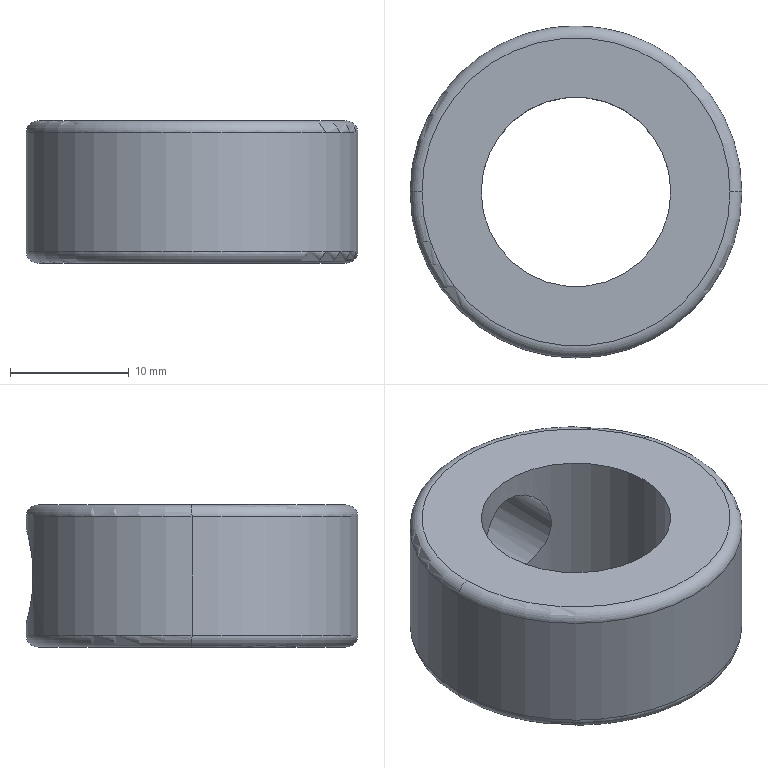Part | SolidWorks | features Extrusion 1, Fillet 1, ICE 1 | 1 solid | 12 faces | box 28 x 28 x 12 mm | volume 4632 mm3 | cylinder 6 | torus 4 | plane 2 | commonest cylinder face diameters 8 x2 16 x2 28 x2
STEP:
#1=CARTESIAN_POINT('',(0.,14.,-4.));
#2=VERTEX_POINT('',#1);
#3=CARTESIAN_POINT('',(0.,14.,4.));
#4=VERTEX_POINT('',#3);
#5=CARTESIAN_POINT('',(0.,14.,-4.));
#6=CARTESIAN_POINT('',(-0.2658,14.,-4.));
#7=CARTESIAN_POINT('',(-0.5269,13.992,-3.974));
#8=CARTESIAN_POINT('',(-1.04,13.964,-3.871));
#9=CARTESIAN_POINT('',(-1.295,13.942,-3.794));
#10=CARTESIAN_POINT('',(-1.779,13.889,-3.592));
#11=CARTESIAN_POINT('',(-2.008,13.857,-3.469));
#12=CARTESIAN_POINT('',(-2.442,13.787,-3.179));
#13=CARTESIAN_POINT('',(-2.646,13.749,-3.011));
#14=CARTESIAN_POINT('',(-3.013,13.673,-2.644));
#15=CARTESIAN_POINT('',(-3.178,13.635,-2.443));
#16=CARTESIAN_POINT('',(-3.47,13.564,-2.007));
#17=CARTESIAN_POINT('',(-3.594,13.531,-1.776));
#18=CARTESIAN_POINT('',(-3.793,13.477,-1.295));
#19=CARTESIAN_POINT('',(-3.871,13.454,-1.042));
#20=CARTESIAN_POINT('',(-3.974,13.424,-0.5247));
#21=CARTESIAN_POINT('',(-4.,13.416,-0.2642));
#22=CARTESIAN_POINT('',(-4.,13.416,0.2607));
#23=CARTESIAN_POINT('',(-3.974,13.424,0.5273));
#24=CARTESIAN_POINT('',(-3.871,13.454,1.042));
#25=CARTESIAN_POINT('',(-3.795,13.476,1.292));
#26=CARTESIAN_POINT('',(-3.593,13.532,1.778));
#27=CARTESIAN_POINT('',(-3.468,13.564,2.009));
#28=CARTESIAN_POINT('',(-3.179,13.635,2.441));
#29=CARTESIAN_POINT('',(-3.012,13.673,2.645));
#30=CARTESIAN_POINT('',(-2.643,13.75,3.014));
#31=CARTESIAN_POINT('',(-2.442,13.787,3.179));
#32=CARTESIAN_POINT('',(-2.01,13.857,3.468));
#33=CARTESIAN_POINT('',(-1.776,13.889,3.594));
#34=CARTESIAN_POINT('',(-1.293,13.942,3.794));
#35=CARTESIAN_POINT('',(-1.044,13.963,3.87));
#36=CARTESIAN_POINT('',(-0.5274,13.992,3.974));
#37=CARTESIAN_POINT('',(-0.2619,14.,4.));
#38=CARTESIAN_POINT('',(0.,14.,4.));
#39=B_SPLINE_CURVE_WITH_KNOTS('',3,(#5,#6,#7,#8,#9,#10,#11,#12,#13,#14,#15,#16,#17,#18,#19,#20,#21,#22,#23,#24,#25,#26,#27,#28,#29,#30,#31,#32,#33,#34,#35,#36,#37,#38),.UNSPECIFIED.,.F.,.F.,(4,2,2,2,2,2,2,2,2,2,2,2,2,2,2,2,4),(0.,0.0007857,0.001571,0.002357,0.003143,0.003929,0.004714,0.0055,0.006286,0.007072,0.007857,0.008643,0.009429,0.01021,0.011,0.01179,0.01257),.UNSPECIFIED.);
#40=EDGE_CURVE('',#2,#4,#39,.T.);
#41=ORIENTED_EDGE('',*,*,#40,.T.);
#42=CARTESIAN_POINT('',(0.,8.,4.));
#43=VERTEX_POINT('',#42);
#44=CARTESIAN_POINT('',(0.,20.,4.));
#45=DIRECTION('',(0.,-1.,0.));
#46=VECTOR('',#45,1000.);
#47=LINE('',#44,#46);
#48=EDGE_CURVE('',#4,#43,#47,.T.);
#49=ORIENTED_EDGE('',*,*,#48,.T.);
#50=CARTESIAN_POINT('',(0.,8.,-4.));
#51=VERTEX_POINT('',#50);
#52=CARTESIAN_POINT('',(0.,8.,-4.));
#53=CARTESIAN_POINT('',(-0.2692,8.,-4.));
#54=CARTESIAN_POINT('',(-0.5331,7.986,-3.973));
#55=CARTESIAN_POINT('',(-1.051,7.935,-3.869));
#56=CARTESIAN_POINT('',(-1.307,7.896,-3.789));
#57=CARTESIAN_POINT('',(-1.79,7.801,-3.587));
#58=CARTESIAN_POINT('',(-2.019,7.744,-3.463));
#59=CARTESIAN_POINT('',(-2.45,7.619,-3.172));
#60=CARTESIAN_POINT('',(-2.65,7.551,-3.007));
#61=CARTESIAN_POINT('',(-3.013,7.414,-2.644));
#62=CARTESIAN_POINT('',(-3.178,7.344,-2.443));
#63=CARTESIAN_POINT('',(-3.466,7.212,-2.013));
#64=CARTESIAN_POINT('',(-3.589,7.151,-1.786));
#65=CARTESIAN_POINT('',(-3.789,7.046,-1.307));
#66=CARTESIAN_POINT('',(-3.869,7.003,-1.051));
#67=CARTESIAN_POINT('',(-3.973,6.944,-0.5326));
#68=CARTESIAN_POINT('',(-4.,6.928,-0.2701));
#69=CARTESIAN_POINT('',(-4.,6.928,0.2623));
#70=CARTESIAN_POINT('',(-3.973,6.944,0.532));
#71=CARTESIAN_POINT('',(-3.869,7.003,1.05));
#72=CARTESIAN_POINT('',(-3.791,7.046,1.304));
#73=CARTESIAN_POINT('',(-3.588,7.151,1.788));
#74=CARTESIAN_POINT('',(-3.465,7.213,2.016));
#75=CARTESIAN_POINT('',(-3.176,7.344,2.445));
#76=CARTESIAN_POINT('',(-3.01,7.415,2.647));
#77=CARTESIAN_POINT('',(-2.647,7.552,3.01));
#78=CARTESIAN_POINT('',(-2.449,7.619,3.173));
#79=CARTESIAN_POINT('',(-2.016,7.745,3.465));
#80=CARTESIAN_POINT('',(-1.786,7.802,3.588));
#81=CARTESIAN_POINT('',(-1.306,7.896,3.79));
#82=CARTESIAN_POINT('',(-1.052,7.935,3.868));
#83=CARTESIAN_POINT('',(-0.5291,7.987,3.974));
#84=CARTESIAN_POINT('',(-0.2656,8.,4.));
#85=CARTESIAN_POINT('',(0.,8.,4.));
#86=B_SPLINE_CURVE_WITH_KNOTS('',3,(#52,#53,#54,#55,#56,#57,#58,#59,#60,#61,#62,#63,#64,#65,#66,#67,#68,#69,#70,#71,#72,#73,#74,#75,#76,#77,#78,#79,#80,#81,#82,#83,#84,#85),.UNSPECIFIED.,.F.,.F.,(4,2,2,2,2,2,2,2,2,2,2,2,2,2,2,2,4),(0.,0.0007952,0.00159,0.002386,0.003181,0.003976,0.004771,0.005567,0.006362,0.007157,0.007952,0.008748,0.009543,0.01034,0.01113,0.01193,0.01272),.UNSPECIFIED.);
#87=EDGE_CURVE('',#51,#43,#86,.T.);
#88=ORIENTED_EDGE('',*,*,#87,.F.);
#89=CARTESIAN_POINT('',(0.,20.,-4.));
#90=DIRECTION('',(0.,-1.,0.));
#91=VECTOR('',#90,1000.);
#92=LINE('',#89,#91);
#93=EDGE_CURVE('',#2,#51,#92,.T.);
#94=ORIENTED_EDGE('',*,*,#93,.F.);
#95=EDGE_LOOP('',(#41,#49,#88,#94));
#96=FACE_OUTER_BOUND('',#95,.T.);
#97=CARTESIAN_POINT('',(0.,20.,0.));
#98=DIRECTION('',(0.,-1.,0.));
#99=DIRECTION('',(0.,0.,-1.));
#100=AXIS2_PLACEMENT_3D('',#97,#98,#99);
#101=CYLINDRICAL_SURFACE('',#100,4.);
#102=ADVANCED_FACE('',(#96),#101,.F.);
#103=CARTESIAN_POINT('',(-14.,0.,5.));
#104=VERTEX_POINT('',#103);
#105=CARTESIAN_POINT('',(14.,0.,5.));
#106=VERTEX_POINT('',#105);
#107=CARTESIAN_POINT('',(0.,0.,5.));
#108=DIRECTION('',(0.,0.,-1.));
#109=DIRECTION('',(1.,0.,0.));
#110=AXIS2_PLACEMENT_3D('',#107,#108,#109);
#111=CIRCLE('',#110,14.);
#112=EDGE_CURVE('',#104,#106,#111,.T.);
#113=ORIENTED_EDGE('',*,*,#112,.F.);
#114=CARTESIAN_POINT('',(-13.,0.,6.));
#115=VERTEX_POINT('',#114);
#116=CARTESIAN_POINT('',(-13.,0.,5.));
#117=DIRECTION('',(0.,1.,0.));
#118=DIRECTION('',(-1.,0.,0.));
#119=AXIS2_PLACEMENT_3D('',#116,#117,#118);
#120=CIRCLE('',#119,1.);
#121=EDGE_CURVE('',#104,#115,#120,.T.);
#122=ORIENTED_EDGE('',*,*,#121,.T.);
#123=CARTESIAN_POINT('',(13.,0.,6.));
#124=VERTEX_POINT('',#123);
#125=CARTESIAN_POINT('',(0.,0.,6.));
#126=DIRECTION('',(0.,0.,1.));
#127=DIRECTION('',(1.,0.,0.));
#128=AXIS2_PLACEMENT_3D('',#125,#126,#127);
#129=CIRCLE('',#128,13.);
#130=EDGE_CURVE('',#124,#115,#129,.T.);
#131=ORIENTED_EDGE('',*,*,#130,.F.);
#132=CARTESIAN_POINT('',(13.,0.,5.));
#133=DIRECTION('',(0.,-1.,0.));
#134=DIRECTION('',(0.,0.,-1.));
#135=AXIS2_PLACEMENT_3D('',#132,#133,#134);
#136=CIRCLE('',#135,1.);
#137=EDGE_CURVE('',#106,#124,#136,.T.);
#138=ORIENTED_EDGE('',*,*,#137,.F.);
#139=EDGE_LOOP('',(#113,#122,#131,#138));
#140=FACE_OUTER_BOUND('',#139,.T.);
#141=CARTESIAN_POINT('',(0.,0.,5.));
#142=DIRECTION('',(0.,0.,1.));
#143=DIRECTION('',(1.,0.,0.));
#144=AXIS2_PLACEMENT_3D('',#141,#142,#143);
#145=TOROIDAL_SURFACE('',#144,13.,1.);
#146=ADVANCED_FACE('',(#140),#145,.T.);
#147=CARTESIAN_POINT('',(-13.,0.,-6.));
#148=VERTEX_POINT('',#147);
#149=CARTESIAN_POINT('',(13.,0.,-6.));
#150=VERTEX_POINT('',#149);
#151=CARTESIAN_POINT('',(0.,0.,-6.));
#152=DIRECTION('',(0.,0.,-1.));
#153=DIRECTION('',(1.,0.,0.));
#154=AXIS2_PLACEMENT_3D('',#151,#152,#153);
#155=CIRCLE('',#154,13.);
#156=EDGE_CURVE('',#148,#150,#155,.T.);
#157=ORIENTED_EDGE('',*,*,#156,.F.);
#158=CARTESIAN_POINT('',(-14.,0.,-5.));
#159=VERTEX_POINT('',#158);
#160=CARTESIAN_POINT('',(-13.,0.,-5.));
#161=DIRECTION('',(0.,1.,0.));
#162=DIRECTION('',(-1.,0.,0.));
#163=AXIS2_PLACEMENT_3D('',#160,#161,#162);
#164=CIRCLE('',#163,1.);
#165=EDGE_CURVE('',#148,#159,#164,.T.);
#166=ORIENTED_EDGE('',*,*,#165,.T.);
#167=CARTESIAN_POINT('',(14.,0.,-5.));
#168=VERTEX_POINT('',#167);
#169=CARTESIAN_POINT('',(0.,0.,-5.));
#170=DIRECTION('',(0.,0.,1.));
#171=DIRECTION('',(1.,0.,0.));
#172=AXIS2_PLACEMENT_3D('',#169,#170,#171);
#173=CIRCLE('',#172,14.);
#174=EDGE_CURVE('',#168,#159,#173,.T.);
#175=ORIENTED_EDGE('',*,*,#174,.F.);
#176=CARTESIAN_POINT('',(13.,0.,-5.));
#177=DIRECTION('',(0.,-1.,0.));
#178=DIRECTION('',(0.,0.,-1.));
#179=AXIS2_PLACEMENT_3D('',#176,#177,#178);
#180=CIRCLE('',#179,1.);
#181=EDGE_CURVE('',#150,#168,#180,.T.);
#182=ORIENTED_EDGE('',*,*,#181,.F.);
#183=EDGE_LOOP('',(#157,#166,#175,#182));
#184=FACE_OUTER_BOUND('',#183,.T.);
#185=CARTESIAN_POINT('',(0.,0.,-5.));
#186=DIRECTION('',(0.,0.,1.));
#187=DIRECTION('',(1.,0.,0.));
#188=AXIS2_PLACEMENT_3D('',#185,#186,#187);
#189=TOROIDAL_SURFACE('',#188,13.,1.);
#190=ADVANCED_FACE('',(#184),#189,.T.);
#191=CARTESIAN_POINT('',(-8.,0.,6.));
#192=VERTEX_POINT('',#191);
#193=CARTESIAN_POINT('',(8.,0.,6.));
#194=VERTEX_POINT('',#193);
#195=CARTESIAN_POINT('',(0.,0.,6.));
#196=DIRECTION('',(0.,0.,1.));
#197=DIRECTION('',(1.,0.,0.));
#198=AXIS2_PLACEMENT_3D('',#195,#196,#197);
#199=CIRCLE('',#198,8.);
#200=EDGE_CURVE('',#192,#194,#199,.T.);
#201=ORIENTED_EDGE('',*,*,#200,.T.);
#202=CARTESIAN_POINT('',(8.,0.,-6.));
#203=VERTEX_POINT('',#202);
#204=CARTESIAN_POINT('',(8.,0.,6.));
#205=DIRECTION('',(0.,0.,-1.));
#206=VECTOR('',#205,1000.);
#207=LINE('',#204,#206);
#208=EDGE_CURVE('',#194,#203,#207,.T.);
#209=ORIENTED_EDGE('',*,*,#208,.T.);
#210=CARTESIAN_POINT('',(-8.,0.,-6.));
#211=VERTEX_POINT('',#210);
#212=CARTESIAN_POINT('',(0.,0.,-6.));
#213=DIRECTION('',(0.,0.,1.));
#214=DIRECTION('',(1.,0.,0.));
#215=AXIS2_PLACEMENT_3D('',#212,#213,#214);
#216=CIRCLE('',#215,8.);
#217=EDGE_CURVE('',#211,#203,#216,.T.);
#218=ORIENTED_EDGE('',*,*,#217,.F.);
#219=CARTESIAN_POINT('',(-8.,0.,6.));
#220=DIRECTION('',(0.,0.,-1.));
#221=VECTOR('',#220,1000.);
#222=LINE('',#219,#221);
#223=EDGE_CURVE('',#192,#211,#222,.T.);
#224=ORIENTED_EDGE('',*,*,#223,.F.);
#225=EDGE_LOOP('',(#201,#209,#218,#224));
#226=FACE_OUTER_BOUND('',#225,.T.);
#227=CARTESIAN_POINT('',(0.,0.,6.));
#228=DIRECTION('',(0.,0.,-1.));
#229=DIRECTION('',(-1.,0.,0.));
#230=AXIS2_PLACEMENT_3D('',#227,#228,#229);
#231=CYLINDRICAL_SURFACE('',#230,8.);
#232=ADVANCED_FACE('',(#226),#231,.F.);
#233=ORIENTED_EDGE('',*,*,#40,.F.);
#234=CARTESIAN_POINT('',(0.,14.,4.));
#235=CARTESIAN_POINT('',(0.2619,14.,4.));
#236=CARTESIAN_POINT('',(0.524,13.993,3.974));
#237=CARTESIAN_POINT('',(1.043,13.963,3.871));
#238=CARTESIAN_POINT('',(1.294,13.942,3.794));
#239=CARTESIAN_POINT('',(1.776,13.889,3.594));
#240=CARTESIAN_POINT('',(2.01,13.857,3.468));
#241=CARTESIAN_POINT('',(2.443,13.787,3.178));
#242=CARTESIAN_POINT('',(2.643,13.749,3.013));
#243=CARTESIAN_POINT('',(3.012,13.673,2.645));
#244=CARTESIAN_POINT('',(3.18,13.635,2.441));
#245=CARTESIAN_POINT('',(3.468,13.564,2.009));
#246=CARTESIAN_POINT('',(3.592,13.532,1.78));
#247=CARTESIAN_POINT('',(3.795,13.476,1.292));
#248=CARTESIAN_POINT('',(3.871,13.454,1.042));
#249=CARTESIAN_POINT('',(3.973,13.424,0.5296));
#250=CARTESIAN_POINT('',(4.,13.416,0.2643));
#251=CARTESIAN_POINT('',(4.,13.416,-0.2631));
#252=CARTESIAN_POINT('',(3.974,13.424,-0.5236));
#253=CARTESIAN_POINT('',(3.872,13.454,-1.038));
#254=CARTESIAN_POINT('',(3.794,13.477,-1.294));
#255=CARTESIAN_POINT('',(3.594,13.531,-1.776));
#256=CARTESIAN_POINT('',(3.471,13.564,-2.005));
#257=CARTESIAN_POINT('',(3.179,13.635,-2.442));
#258=CARTESIAN_POINT('',(3.013,13.673,-2.644));
#259=CARTESIAN_POINT('',(2.646,13.749,-3.011));
#260=CARTESIAN_POINT('',(2.443,13.787,-3.178));
#261=CARTESIAN_POINT('',(2.008,13.857,-3.469));
#262=CARTESIAN_POINT('',(1.779,13.889,-3.592));
#263=CARTESIAN_POINT('',(1.297,13.942,-3.793));
#264=CARTESIAN_POINT('',(1.042,13.964,-3.871));
#265=CARTESIAN_POINT('',(0.5273,13.992,-3.974));
#266=CARTESIAN_POINT('',(0.2657,14.,-4.));
#267=CARTESIAN_POINT('',(0.,14.,-4.));
#268=B_SPLINE_CURVE_WITH_KNOTS('',3,(#234,#235,#236,#237,#238,#239,#240,#241,#242,#243,#244,#245,#246,#247,#248,#249,#250,#251,#252,#253,#254,#255,#256,#257,#258,#259,#260,#261,#262,#263,#264,#265,#266,#267),.UNSPECIFIED.,.F.,.F.,(4,2,2,2,2,2,2,2,2,2,2,2,2,2,2,2,4),(0.01257,0.01336,0.01414,0.01493,0.01571,0.0165,0.01728,0.01807,0.01886,0.01964,0.02043,0.02121,0.022,0.02278,0.02357,0.02435,0.02514),.UNSPECIFIED.);
#269=EDGE_CURVE('',#4,#2,#268,.T.);
#270=ORIENTED_EDGE('',*,*,#269,.F.);
#271=EDGE_LOOP('',(#233,#270));
#272=FACE_BOUND('',#271,.T.);
#273=ORIENTED_EDGE('',*,*,#112,.T.);
#274=CARTESIAN_POINT('',(14.,0.,6.));
#275=DIRECTION('',(0.,0.,-1.));
#276=VECTOR('',#275,1000.);
#277=LINE('',#274,#276);
#278=EDGE_CURVE('',#106,#168,#277,.T.);
#279=ORIENTED_EDGE('',*,*,#278,.T.);
#280=ORIENTED_EDGE('',*,*,#174,.T.);
#281=CARTESIAN_POINT('',(-14.,0.,6.));
#282=DIRECTION('',(0.,0.,-1.));
#283=VECTOR('',#282,1000.);
#284=LINE('',#281,#283);
#285=EDGE_CURVE('',#104,#159,#284,.T.);
#286=ORIENTED_EDGE('',*,*,#285,.F.);
#287=EDGE_LOOP('',(#273,#279,#280,#286));
#288=FACE_OUTER_BOUND('',#287,.T.);
#289=CARTESIAN_POINT('',(0.,0.,6.));
#290=DIRECTION('',(0.,0.,-1.));
#291=DIRECTION('',(-1.,0.,0.));
#292=AXIS2_PLACEMENT_3D('',#289,#290,#291);
#293=CYLINDRICAL_SURFACE('',#292,14.);
#294=ADVANCED_FACE('',(#272,#288),#293,.T.);
#295=ORIENTED_EDGE('',*,*,#278,.F.);
#296=CARTESIAN_POINT('',(0.,0.,5.));
#297=DIRECTION('',(0.,0.,-1.));
#298=DIRECTION('',(1.,0.,0.));
#299=AXIS2_PLACEMENT_3D('',#296,#297,#298);
#300=CIRCLE('',#299,14.);
#301=EDGE_CURVE('',#106,#104,#300,.T.);
#302=ORIENTED_EDGE('',*,*,#301,.T.);
#303=ORIENTED_EDGE('',*,*,#285,.T.);
#304=CARTESIAN_POINT('',(0.,0.,-5.));
#305=DIRECTION('',(0.,0.,1.));
#306=DIRECTION('',(1.,0.,0.));
#307=AXIS2_PLACEMENT_3D('',#304,#305,#306);
#308=CIRCLE('',#307,14.);
#309=EDGE_CURVE('',#159,#168,#308,.T.);
#310=ORIENTED_EDGE('',*,*,#309,.T.);
#311=EDGE_LOOP('',(#295,#302,#303,#310));
#312=FACE_OUTER_BOUND('',#311,.T.);
#313=CARTESIAN_POINT('',(0.,0.,6.));
#314=DIRECTION('',(0.,0.,-1.));
#315=DIRECTION('',(-1.,0.,0.));
#316=AXIS2_PLACEMENT_3D('',#313,#314,#315);
#317=CYLINDRICAL_SURFACE('',#316,14.);
#318=ADVANCED_FACE('',(#312),#317,.T.);
#319=ORIENTED_EDGE('',*,*,#208,.F.);
#320=CARTESIAN_POINT('',(0.,0.,6.));
#321=DIRECTION('',(0.,0.,1.));
#322=DIRECTION('',(1.,0.,0.));
#323=AXIS2_PLACEMENT_3D('',#320,#321,#322);
#324=CIRCLE('',#323,8.);
#325=EDGE_CURVE('',#194,#192,#324,.T.);
#326=ORIENTED_EDGE('',*,*,#325,.T.);
#327=ORIENTED_EDGE('',*,*,#223,.T.);
#328=CARTESIAN_POINT('',(0.,0.,-6.));
#329=DIRECTION('',(0.,0.,1.));
#330=DIRECTION('',(1.,0.,0.));
#331=AXIS2_PLACEMENT_3D('',#328,#329,#330);
#332=CIRCLE('',#331,8.);
#333=EDGE_CURVE('',#203,#211,#332,.T.);
#334=ORIENTED_EDGE('',*,*,#333,.F.);
#335=EDGE_LOOP('',(#319,#326,#327,#334));
#336=FACE_OUTER_BOUND('',#335,.T.);
#337=ORIENTED_EDGE('',*,*,#87,.T.);
#338=CARTESIAN_POINT('',(0.,8.,4.));
#339=CARTESIAN_POINT('',(0.2651,8.,4.));
#340=CARTESIAN_POINT('',(0.5349,7.986,3.973));
#341=CARTESIAN_POINT('',(1.053,7.935,3.868));
#342=CARTESIAN_POINT('',(1.305,7.897,3.79));
#343=CARTESIAN_POINT('',(1.792,7.801,3.586));
#344=CARTESIAN_POINT('',(2.021,7.744,3.462));
#345=CARTESIAN_POINT('',(2.449,7.619,3.173));
#346=CARTESIAN_POINT('',(2.651,7.551,3.006));
#347=CARTESIAN_POINT('',(3.014,7.413,2.642));
#348=CARTESIAN_POINT('',(3.176,7.344,2.445));
#349=CARTESIAN_POINT('',(3.465,7.213,2.016));
#350=CARTESIAN_POINT('',(3.589,7.151,1.785));
#351=CARTESIAN_POINT('',(3.79,7.046,1.306));
#352=CARTESIAN_POINT('',(3.867,7.004,1.057));
#353=CARTESIAN_POINT('',(3.973,6.944,0.5351));
#354=CARTESIAN_POINT('',(4.,6.928,0.2689));
#355=CARTESIAN_POINT('',(4.,6.928,-0.1279));
#356=CARTESIAN_POINT('',(3.994,6.932,-0.2603));
#357=CARTESIAN_POINT('',(3.968,6.947,-0.5254));
#358=CARTESIAN_POINT('',(3.948,6.958,-0.6587));
#359=CARTESIAN_POINT('',(3.869,7.002,-1.049));
#360=CARTESIAN_POINT('',(3.792,7.045,-1.3));
#361=CARTESIAN_POINT('',(3.59,7.15,-1.784));
#362=CARTESIAN_POINT('',(3.465,7.212,-2.014));
#363=CARTESIAN_POINT('',(3.178,7.343,-2.442));
#364=CARTESIAN_POINT('',(3.013,7.413,-2.643));
#365=CARTESIAN_POINT('',(2.649,7.551,-3.009));
#366=CARTESIAN_POINT('',(2.451,7.619,-3.172));
#367=CARTESIAN_POINT('',(2.023,7.743,-3.46));
#368=CARTESIAN_POINT('',(1.79,7.801,-3.587));
#369=CARTESIAN_POINT('',(1.308,7.896,-3.789));
#370=CARTESIAN_POINT('',(1.058,7.934,-3.867));
#371=CARTESIAN_POINT('',(0.5388,7.986,-3.972));
#372=CARTESIAN_POINT('',(0.2687,8.,-4.));
#373=CARTESIAN_POINT('',(0.,8.,-4.));
#374=B_SPLINE_CURVE_WITH_KNOTS('',3,(#338,#339,#340,#341,#342,#343,#344,#345,#346,#347,#348,#349,#350,#351,#352,#353,#354,#355,#356,#357,#358,#359,#360,#361,#362,#363,#364,#365,#366,#367,#368,#369,#370,#371,#372,#373),.UNSPECIFIED.,.F.,.F.,(4,2,2,2,2,2,2,2,2,2,2,2,2,2,2,2,2,4),(0.01272,0.01352,0.01431,0.01511,0.0159,0.01669,0.01749,0.01828,0.01907,0.01947,0.01987,0.02066,0.02146,0.02225,0.02304,0.02384,0.02463,0.02543),.UNSPECIFIED.);
#375=EDGE_CURVE('',#43,#51,#374,.T.);
#376=ORIENTED_EDGE('',*,*,#375,.T.);
#377=EDGE_LOOP('',(#337,#376));
#378=FACE_BOUND('',#377,.T.);
#379=CARTESIAN_POINT('',(0.,0.,6.));
#380=DIRECTION('',(0.,0.,-1.));
#381=DIRECTION('',(-1.,0.,0.));
#382=AXIS2_PLACEMENT_3D('',#379,#380,#381);
#383=CYLINDRICAL_SURFACE('',#382,8.);
#384=ADVANCED_FACE('',(#336,#378),#383,.F.);
#385=ORIENTED_EDGE('',*,*,#130,.T.);
#386=CARTESIAN_POINT('',(0.,0.,6.));
#387=DIRECTION('',(0.,0.,1.));
#388=DIRECTION('',(1.,0.,0.));
#389=AXIS2_PLACEMENT_3D('',#386,#387,#388);
#390=CIRCLE('',#389,13.);
#391=EDGE_CURVE('',#115,#124,#390,.T.);
#392=ORIENTED_EDGE('',*,*,#391,.T.);
#393=EDGE_LOOP('',(#385,#392));
#394=FACE_OUTER_BOUND('',#393,.T.);
#395=ORIENTED_EDGE('',*,*,#200,.F.);
#396=ORIENTED_EDGE('',*,*,#325,.F.);
#397=EDGE_LOOP('',(#395,#396));
#398=FACE_BOUND('',#397,.T.);
#399=CARTESIAN_POINT('',(0.,0.,6.));
#400=DIRECTION('',(0.,0.,1.));
#401=DIRECTION('',(1.,0.,0.));
#402=AXIS2_PLACEMENT_3D('',#399,#400,#401);
#403=PLANE('',#402);
#404=ADVANCED_FACE('',(#394,#398),#403,.T.);
#405=CARTESIAN_POINT('',(0.,0.,-6.));
#406=DIRECTION('',(0.,0.,-1.));
#407=DIRECTION('',(1.,0.,0.));
#408=AXIS2_PLACEMENT_3D('',#405,#406,#407);
#409=CIRCLE('',#408,13.);
#410=EDGE_CURVE('',#150,#148,#409,.T.);
#411=ORIENTED_EDGE('',*,*,#410,.T.);
#412=ORIENTED_EDGE('',*,*,#156,.T.);
#413=EDGE_LOOP('',(#411,#412));
#414=FACE_OUTER_BOUND('',#413,.T.);
#415=ORIENTED_EDGE('',*,*,#217,.T.);
#416=ORIENTED_EDGE('',*,*,#333,.T.);
#417=EDGE_LOOP('',(#415,#416));
#418=FACE_BOUND('',#417,.T.);
#419=CARTESIAN_POINT('',(0.,0.,-6.));
#420=DIRECTION('',(0.,0.,1.));
#421=DIRECTION('',(1.,0.,0.));
#422=AXIS2_PLACEMENT_3D('',#419,#420,#421);
#423=PLANE('',#422);
#424=ADVANCED_FACE('',(#414,#418),#423,.F.);
#425=ORIENTED_EDGE('',*,*,#165,.F.);
#426=ORIENTED_EDGE('',*,*,#410,.F.);
#427=ORIENTED_EDGE('',*,*,#181,.T.);
#428=ORIENTED_EDGE('',*,*,#309,.F.);
#429=EDGE_LOOP('',(#425,#426,#427,#428));
#430=FACE_OUTER_BOUND('',#429,.T.);
#431=CARTESIAN_POINT('',(0.,0.,-5.));
#432=DIRECTION('',(0.,0.,1.));
#433=DIRECTION('',(1.,0.,0.));
#434=AXIS2_PLACEMENT_3D('',#431,#432,#433);
#435=TOROIDAL_SURFACE('',#434,13.,1.);
#436=ADVANCED_FACE('',(#430),#435,.T.);
#437=ORIENTED_EDGE('',*,*,#121,.F.);
#438=ORIENTED_EDGE('',*,*,#301,.F.);
#439=ORIENTED_EDGE('',*,*,#137,.T.);
#440=ORIENTED_EDGE('',*,*,#391,.F.);
#441=EDGE_LOOP('',(#437,#438,#439,#440));
#442=FACE_OUTER_BOUND('',#441,.T.);
#443=CARTESIAN_POINT('',(0.,0.,5.));
#444=DIRECTION('',(0.,0.,1.));
#445=DIRECTION('',(1.,0.,0.));
#446=AXIS2_PLACEMENT_3D('',#443,#444,#445);
#447=TOROIDAL_SURFACE('',#446,13.,1.);
#448=ADVANCED_FACE('',(#442),#447,.T.);
#449=ORIENTED_EDGE('',*,*,#48,.F.);
#450=ORIENTED_EDGE('',*,*,#269,.T.);
#451=ORIENTED_EDGE('',*,*,#93,.T.);
#452=ORIENTED_EDGE('',*,*,#375,.F.);
#453=EDGE_LOOP('',(#449,#450,#451,#452));
#454=FACE_OUTER_BOUND('',#453,.T.);
#455=CARTESIAN_POINT('',(0.,20.,0.));
#456=DIRECTION('',(0.,-1.,0.));
#457=DIRECTION('',(0.,0.,-1.));
#458=AXIS2_PLACEMENT_3D('',#455,#456,#457);
#459=CYLINDRICAL_SURFACE('',#458,4.);
#460=ADVANCED_FACE('',(#454),#459,.F.);
#461=CLOSED_SHELL('',(#102,#146,#190,#232,#294,#318,#384,#404,#424,#436,#448,#460));
#462=MANIFOLD_SOLID_BREP('',#461);
#463=CARTESIAN_POINT('',(0.,0.,0.));
#464=DIRECTION('',(0.,0.,1.));
#465=DIRECTION('',(1.,0.,0.));
#466=AXIS2_PLACEMENT_3D('',#463,#464,#465);
#467=(LENGTH_UNIT()NAMED_UNIT(*)SI_UNIT(.MILLI.,.METRE.));
#468=UNCERTAINTY_MEASURE_WITH_UNIT(LENGTH_MEASURE(0.00001),#467,'','');
#469=(NAMED_UNIT(*)PLANE_ANGLE_UNIT()SI_UNIT($,.RADIAN.));
#470=(NAMED_UNIT(*)SI_UNIT($,.STERADIAN.)SOLID_ANGLE_UNIT());
#471=(GEOMETRIC_REPRESENTATION_CONTEXT(3)GLOBAL_UNCERTAINTY_ASSIGNED_CONTEXT((#468))GLOBAL_UNIT_ASSIGNED_CONTEXT((#467,#469,#470))REPRESENTATION_CONTEXT('',''));
#472=ADVANCED_BREP_SHAPE_REPRESENTATION('',(#462,#466),#471);